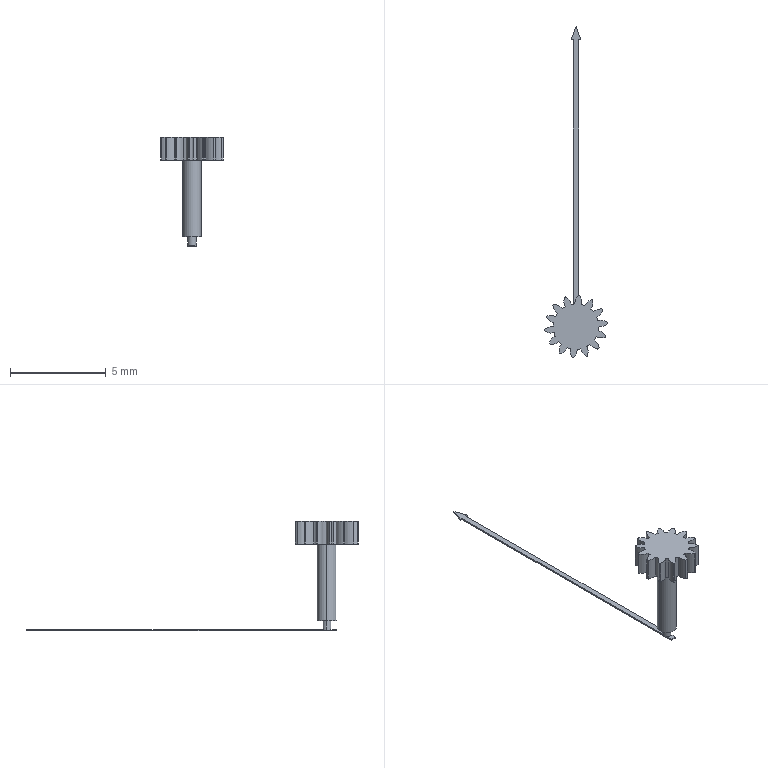Part | SolidWorks | features ICE 5, CirPattern 1, Extrusion 1 | 1 solid | 75 faces | box 3.258 x 17.347 x 5.736 mm | volume 10.917 mm3 | cylinder 32 | spline 28 | plane 15 | commonest cylinder face diameters 2.376 x14 3.276 x14 0.439 x2 1 x2